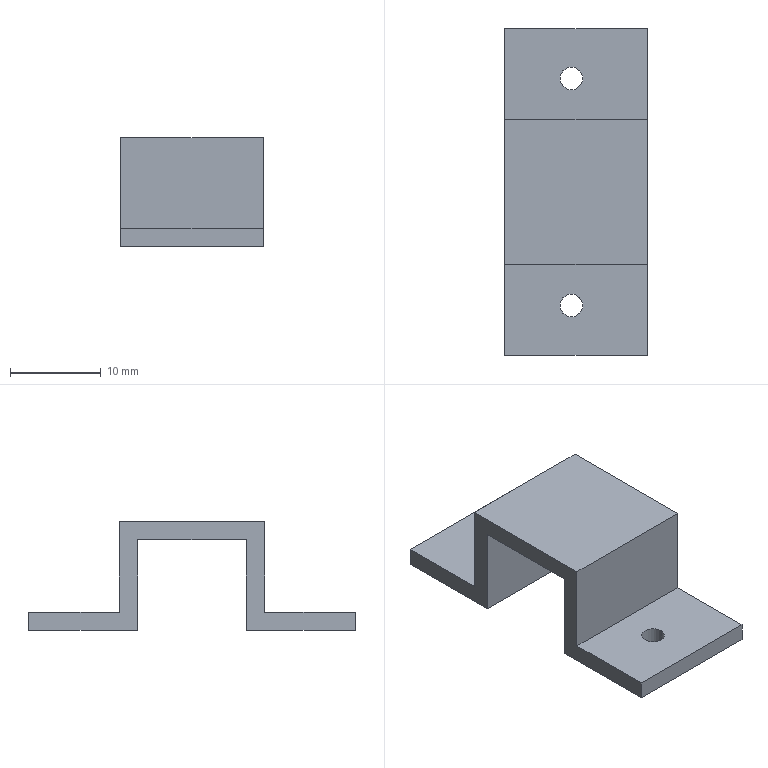Part | SolidWorks | features ICE 3, Extrusion 1, HoleWzd 1 | 1 solid | 18 faces | box 15.7 x 36 x 12 mm | volume 1739 mm3 | plane 14 | cylinder 4 | commonest cylinder face diameters 2.5 x4
STEP:
#1=CARTESIAN_POINT('',(1.25,-12.5,-10.));
#2=VERTEX_POINT('',#1);
#3=CARTESIAN_POINT('',(-1.25,-12.5,-10.));
#4=VERTEX_POINT('',#3);
#5=CARTESIAN_POINT('',(0.,-12.5,-10.));
#6=DIRECTION('',(0.,0.,-1.));
#7=DIRECTION('',(-1.,0.,0.));
#8=AXIS2_PLACEMENT_3D('',#5,#6,#7);
#9=CIRCLE('',#8,1.25);
#10=EDGE_CURVE('',#2,#4,#9,.T.);
#11=ORIENTED_EDGE('',*,*,#10,.T.);
#12=CARTESIAN_POINT('',(-1.25,-12.5,-8.));
#13=VERTEX_POINT('',#12);
#14=CARTESIAN_POINT('',(-1.25,-12.5,-8.));
#15=DIRECTION('',(0.,0.,1.));
#16=VECTOR('',#15,1000.);
#17=LINE('',#14,#16);
#18=EDGE_CURVE('',#4,#13,#17,.T.);
#19=ORIENTED_EDGE('',*,*,#18,.T.);
#20=CARTESIAN_POINT('',(1.25,-12.5,-8.));
#21=VERTEX_POINT('',#20);
#22=CARTESIAN_POINT('',(0.,-12.5,-8.));
#23=DIRECTION('',(0.,0.,1.));
#24=DIRECTION('',(1.,0.,0.));
#25=AXIS2_PLACEMENT_3D('',#22,#23,#24);
#26=CIRCLE('',#25,1.25);
#27=EDGE_CURVE('',#13,#21,#26,.T.);
#28=ORIENTED_EDGE('',*,*,#27,.T.);
#29=CARTESIAN_POINT('',(1.25,-12.5,-8.));
#30=DIRECTION('',(0.,0.,1.));
#31=VECTOR('',#30,1000.);
#32=LINE('',#29,#31);
#33=EDGE_CURVE('',#2,#21,#32,.T.);
#34=ORIENTED_EDGE('',*,*,#33,.F.);
#35=EDGE_LOOP('',(#11,#19,#28,#34));
#36=FACE_OUTER_BOUND('',#35,.T.);
#37=CARTESIAN_POINT('',(0.,-12.5,-8.));
#38=DIRECTION('',(0.,0.,1.));
#39=DIRECTION('',(1.,0.,0.));
#40=AXIS2_PLACEMENT_3D('',#37,#38,#39);
#41=CYLINDRICAL_SURFACE('',#40,1.25);
#42=ADVANCED_FACE('',(#36),#41,.F.);
#43=CARTESIAN_POINT('',(-1.25,12.5,-10.));
#44=VERTEX_POINT('',#43);
#45=CARTESIAN_POINT('',(1.25,12.5,-10.));
#46=VERTEX_POINT('',#45);
#47=CARTESIAN_POINT('',(0.,12.5,-10.));
#48=DIRECTION('',(0.,0.,1.));
#49=DIRECTION('',(1.,0.,0.));
#50=AXIS2_PLACEMENT_3D('',#47,#48,#49);
#51=CIRCLE('',#50,1.25);
#52=EDGE_CURVE('',#44,#46,#51,.T.);
#53=ORIENTED_EDGE('',*,*,#52,.F.);
#54=CARTESIAN_POINT('',(-1.25,12.5,-8.));
#55=VERTEX_POINT('',#54);
#56=CARTESIAN_POINT('',(-1.25,12.5,-8.));
#57=DIRECTION('',(0.,0.,1.));
#58=VECTOR('',#57,1000.);
#59=LINE('',#56,#58);
#60=EDGE_CURVE('',#44,#55,#59,.T.);
#61=ORIENTED_EDGE('',*,*,#60,.T.);
#62=CARTESIAN_POINT('',(1.25,12.5,-8.));
#63=VERTEX_POINT('',#62);
#64=CARTESIAN_POINT('',(0.,12.5,-8.));
#65=DIRECTION('',(0.,0.,1.));
#66=DIRECTION('',(1.,0.,0.));
#67=AXIS2_PLACEMENT_3D('',#64,#65,#66);
#68=CIRCLE('',#67,1.25);
#69=EDGE_CURVE('',#55,#63,#68,.T.);
#70=ORIENTED_EDGE('',*,*,#69,.T.);
#71=CARTESIAN_POINT('',(1.25,12.5,-8.));
#72=DIRECTION('',(0.,0.,1.));
#73=VECTOR('',#72,1000.);
#74=LINE('',#71,#73);
#75=EDGE_CURVE('',#46,#63,#74,.T.);
#76=ORIENTED_EDGE('',*,*,#75,.F.);
#77=EDGE_LOOP('',(#53,#61,#70,#76));
#78=FACE_OUTER_BOUND('',#77,.T.);
#79=CARTESIAN_POINT('',(0.,12.5,-8.));
#80=DIRECTION('',(0.,0.,1.));
#81=DIRECTION('',(1.,0.,0.));
#82=AXIS2_PLACEMENT_3D('',#79,#80,#81);
#83=CYLINDRICAL_SURFACE('',#82,1.25);
#84=ADVANCED_FACE('',(#78),#83,.F.);
#85=CARTESIAN_POINT('',(-7.35,8.,2.));
#86=VERTEX_POINT('',#85);
#87=CARTESIAN_POINT('',(-7.35,8.,-8.));
#88=VERTEX_POINT('',#87);
#89=CARTESIAN_POINT('',(-7.35,8.,2.));
#90=DIRECTION('',(0.,0.,-1.));
#91=VECTOR('',#90,1000.);
#92=LINE('',#89,#91);
#93=EDGE_CURVE('',#86,#88,#92,.T.);
#94=ORIENTED_EDGE('',*,*,#93,.F.);
#95=CARTESIAN_POINT('',(8.35,8.,2.));
#96=VERTEX_POINT('',#95);
#97=CARTESIAN_POINT('',(8.35,8.,2.));
#98=DIRECTION('',(-1.,0.,0.));
#99=VECTOR('',#98,1000.);
#100=LINE('',#97,#99);
#101=EDGE_CURVE('',#96,#86,#100,.T.);
#102=ORIENTED_EDGE('',*,*,#101,.F.);
#103=CARTESIAN_POINT('',(8.35,8.,-8.));
#104=VERTEX_POINT('',#103);
#105=CARTESIAN_POINT('',(8.35,8.,-10.));
#106=DIRECTION('',(0.,0.,1.));
#107=VECTOR('',#106,1000.);
#108=LINE('',#105,#107);
#109=EDGE_CURVE('',#104,#96,#108,.T.);
#110=ORIENTED_EDGE('',*,*,#109,.F.);
#111=CARTESIAN_POINT('',(18.548,8.,-8.));
#112=DIRECTION('',(-1.,0.,0.));
#113=VECTOR('',#112,1000.);
#114=LINE('',#111,#113);
#115=EDGE_CURVE('',#104,#88,#114,.T.);
#116=ORIENTED_EDGE('',*,*,#115,.T.);
#117=EDGE_LOOP('',(#94,#102,#110,#116));
#118=FACE_OUTER_BOUND('',#117,.T.);
#119=CARTESIAN_POINT('',(8.35,8.,-10.));
#120=DIRECTION('',(0.,1.,0.));
#121=DIRECTION('',(0.,0.,1.));
#122=AXIS2_PLACEMENT_3D('',#119,#120,#121);
#123=PLANE('',#122);
#124=ADVANCED_FACE('',(#118),#123,.T.);
#125=CARTESIAN_POINT('',(8.35,-6.,0.));
#126=VERTEX_POINT('',#125);
#127=CARTESIAN_POINT('',(8.35,6.,0.));
#128=VERTEX_POINT('',#127);
#129=CARTESIAN_POINT('',(8.35,6.,0.));
#130=DIRECTION('',(0.,1.,0.));
#131=VECTOR('',#130,1000.);
#132=LINE('',#129,#131);
#133=EDGE_CURVE('',#126,#128,#132,.T.);
#134=ORIENTED_EDGE('',*,*,#133,.T.);
#135=CARTESIAN_POINT('',(8.35,6.,-10.));
#136=VERTEX_POINT('',#135);
#137=CARTESIAN_POINT('',(8.35,6.,-10.));
#138=DIRECTION('',(0.,0.,1.));
#139=VECTOR('',#138,1000.);
#140=LINE('',#137,#139);
#141=EDGE_CURVE('',#136,#128,#140,.T.);
#142=ORIENTED_EDGE('',*,*,#141,.F.);
#143=CARTESIAN_POINT('',(8.35,18.,-10.));
#144=VERTEX_POINT('',#143);
#145=CARTESIAN_POINT('',(8.35,6.,-10.));
#146=DIRECTION('',(0.,1.,0.));
#147=VECTOR('',#146,1000.);
#148=LINE('',#145,#147);
#149=EDGE_CURVE('',#136,#144,#148,.T.);
#150=ORIENTED_EDGE('',*,*,#149,.T.);
#151=CARTESIAN_POINT('',(8.35,18.,-8.));
#152=VERTEX_POINT('',#151);
#153=CARTESIAN_POINT('',(8.35,18.,-10.));
#154=DIRECTION('',(0.,0.,1.));
#155=VECTOR('',#154,1000.);
#156=LINE('',#153,#155);
#157=EDGE_CURVE('',#144,#152,#156,.T.);
#158=ORIENTED_EDGE('',*,*,#157,.T.);
#159=CARTESIAN_POINT('',(8.35,18.,-8.));
#160=DIRECTION('',(0.,-1.,0.));
#161=VECTOR('',#160,1000.);
#162=LINE('',#159,#161);
#163=EDGE_CURVE('',#152,#104,#162,.T.);
#164=ORIENTED_EDGE('',*,*,#163,.T.);
#165=ORIENTED_EDGE('',*,*,#109,.T.);
#166=CARTESIAN_POINT('',(8.35,-8.,2.));
#167=VERTEX_POINT('',#166);
#168=CARTESIAN_POINT('',(8.35,6.,2.));
#169=DIRECTION('',(0.,1.,0.));
#170=VECTOR('',#169,1000.);
#171=LINE('',#168,#170);
#172=EDGE_CURVE('',#167,#96,#171,.T.);
#173=ORIENTED_EDGE('',*,*,#172,.F.);
#174=CARTESIAN_POINT('',(8.35,-8.,-8.));
#175=VERTEX_POINT('',#174);
#176=CARTESIAN_POINT('',(8.35,-8.,-10.));
#177=DIRECTION('',(0.,0.,1.));
#178=VECTOR('',#177,1000.);
#179=LINE('',#176,#178);
#180=EDGE_CURVE('',#175,#167,#179,.T.);
#181=ORIENTED_EDGE('',*,*,#180,.F.);
#182=CARTESIAN_POINT('',(8.35,-18.,-8.));
#183=VERTEX_POINT('',#182);
#184=CARTESIAN_POINT('',(8.35,-18.,-8.));
#185=DIRECTION('',(0.,-1.,0.));
#186=VECTOR('',#185,1000.);
#187=LINE('',#184,#186);
#188=EDGE_CURVE('',#175,#183,#187,.T.);
#189=ORIENTED_EDGE('',*,*,#188,.T.);
#190=CARTESIAN_POINT('',(8.35,-18.,-10.));
#191=VERTEX_POINT('',#190);
#192=CARTESIAN_POINT('',(8.35,-18.,-10.));
#193=DIRECTION('',(0.,0.,-1.));
#194=VECTOR('',#193,1000.);
#195=LINE('',#192,#194);
#196=EDGE_CURVE('',#183,#191,#195,.T.);
#197=ORIENTED_EDGE('',*,*,#196,.T.);
#198=CARTESIAN_POINT('',(8.35,-6.,-10.));
#199=VERTEX_POINT('',#198);
#200=CARTESIAN_POINT('',(8.35,-6.,-10.));
#201=DIRECTION('',(0.,1.,0.));
#202=VECTOR('',#201,1000.);
#203=LINE('',#200,#202);
#204=EDGE_CURVE('',#191,#199,#203,.T.);
#205=ORIENTED_EDGE('',*,*,#204,.T.);
#206=CARTESIAN_POINT('',(8.35,-6.,-10.));
#207=DIRECTION('',(0.,0.,1.));
#208=VECTOR('',#207,1000.);
#209=LINE('',#206,#208);
#210=EDGE_CURVE('',#199,#126,#209,.T.);
#211=ORIENTED_EDGE('',*,*,#210,.T.);
#212=EDGE_LOOP('',(#134,#142,#150,#158,#164,#165,#173,#181,#189,#197,#205,#211));
#213=FACE_OUTER_BOUND('',#212,.T.);
#214=CARTESIAN_POINT('',(8.35,6.,2.));
#215=DIRECTION('',(-1.,0.,0.));
#216=DIRECTION('',(0.,0.,1.));
#217=AXIS2_PLACEMENT_3D('',#214,#215,#216);
#218=PLANE('',#217);
#219=ADVANCED_FACE('',(#213),#218,.F.);
#220=CARTESIAN_POINT('',(-7.35,-8.,2.));
#221=VERTEX_POINT('',#220);
#222=CARTESIAN_POINT('',(-7.35,-8.,2.));
#223=DIRECTION('',(0.,1.,0.));
#224=VECTOR('',#223,1000.);
#225=LINE('',#222,#224);
#226=EDGE_CURVE('',#221,#86,#225,.T.);
#227=ORIENTED_EDGE('',*,*,#226,.F.);
#228=CARTESIAN_POINT('',(8.35,-8.,2.));
#229=DIRECTION('',(1.,0.,0.));
#230=VECTOR('',#229,1000.);
#231=LINE('',#228,#230);
#232=EDGE_CURVE('',#221,#167,#231,.T.);
#233=ORIENTED_EDGE('',*,*,#232,.T.);
#234=ORIENTED_EDGE('',*,*,#172,.T.);
#235=ORIENTED_EDGE('',*,*,#101,.T.);
#236=EDGE_LOOP('',(#227,#233,#234,#235));
#237=FACE_OUTER_BOUND('',#236,.T.);
#238=CARTESIAN_POINT('',(0.,0.,2.));
#239=DIRECTION('',(0.,0.,1.));
#240=DIRECTION('',(1.,0.,0.));
#241=AXIS2_PLACEMENT_3D('',#238,#239,#240);
#242=PLANE('',#241);
#243=ADVANCED_FACE('',(#237),#242,.T.);
#244=CARTESIAN_POINT('',(-7.35,-6.,0.));
#245=VERTEX_POINT('',#244);
#246=CARTESIAN_POINT('',(-8.35,-6.,0.));
#247=DIRECTION('',(1.,0.,0.));
#248=VECTOR('',#247,1000.);
#249=LINE('',#246,#248);
#250=EDGE_CURVE('',#245,#126,#249,.T.);
#251=ORIENTED_EDGE('',*,*,#250,.F.);
#252=CARTESIAN_POINT('',(-7.35,6.,0.));
#253=VERTEX_POINT('',#252);
#254=CARTESIAN_POINT('',(-7.35,6.,0.));
#255=DIRECTION('',(0.,-1.,0.));
#256=VECTOR('',#255,1000.);
#257=LINE('',#254,#256);
#258=EDGE_CURVE('',#253,#245,#257,.T.);
#259=ORIENTED_EDGE('',*,*,#258,.F.);
#260=CARTESIAN_POINT('',(-8.35,6.,0.));
#261=DIRECTION('',(-1.,0.,0.));
#262=VECTOR('',#261,1000.);
#263=LINE('',#260,#262);
#264=EDGE_CURVE('',#128,#253,#263,.T.);
#265=ORIENTED_EDGE('',*,*,#264,.F.);
#266=ORIENTED_EDGE('',*,*,#133,.F.);
#267=EDGE_LOOP('',(#251,#259,#265,#266));
#268=FACE_OUTER_BOUND('',#267,.T.);
#269=CARTESIAN_POINT('',(0.,0.,0.));
#270=DIRECTION('',(0.,0.,1.));
#271=DIRECTION('',(1.,0.,0.));
#272=AXIS2_PLACEMENT_3D('',#269,#270,#271);
#273=PLANE('',#272);
#274=ADVANCED_FACE('',(#268),#273,.F.);
#275=CARTESIAN_POINT('',(-7.35,6.,-10.));
#276=VERTEX_POINT('',#275);
#277=CARTESIAN_POINT('',(-7.35,6.,-10.));
#278=DIRECTION('',(0.,0.,1.));
#279=VECTOR('',#278,1000.);
#280=LINE('',#277,#279);
#281=EDGE_CURVE('',#276,#253,#280,.T.);
#282=ORIENTED_EDGE('',*,*,#281,.F.);
#283=CARTESIAN_POINT('',(-8.35,6.,-10.));
#284=DIRECTION('',(1.,0.,0.));
#285=VECTOR('',#284,1000.);
#286=LINE('',#283,#285);
#287=EDGE_CURVE('',#276,#136,#286,.T.);
#288=ORIENTED_EDGE('',*,*,#287,.T.);
#289=ORIENTED_EDGE('',*,*,#141,.T.);
#290=ORIENTED_EDGE('',*,*,#264,.T.);
#291=EDGE_LOOP('',(#282,#288,#289,#290));
#292=FACE_OUTER_BOUND('',#291,.T.);
#293=CARTESIAN_POINT('',(-8.35,6.,-10.));
#294=DIRECTION('',(0.,-1.,0.));
#295=DIRECTION('',(0.,0.,-1.));
#296=AXIS2_PLACEMENT_3D('',#293,#294,#295);
#297=PLANE('',#296);
#298=ADVANCED_FACE('',(#292),#297,.T.);
#299=CARTESIAN_POINT('',(0.,12.5,-10.));
#300=DIRECTION('',(0.,0.,1.));
#301=DIRECTION('',(1.,0.,0.));
#302=AXIS2_PLACEMENT_3D('',#299,#300,#301);
#303=CIRCLE('',#302,1.25);
#304=EDGE_CURVE('',#46,#44,#303,.T.);
#305=ORIENTED_EDGE('',*,*,#304,.T.);
#306=ORIENTED_EDGE('',*,*,#52,.T.);
#307=EDGE_LOOP('',(#305,#306));
#308=FACE_BOUND('',#307,.T.);
#309=ORIENTED_EDGE('',*,*,#287,.F.);
#310=CARTESIAN_POINT('',(-7.35,18.,-10.));
#311=VERTEX_POINT('',#310);
#312=CARTESIAN_POINT('',(-7.35,18.,-10.));
#313=DIRECTION('',(0.,-1.,0.));
#314=VECTOR('',#313,1000.);
#315=LINE('',#312,#314);
#316=EDGE_CURVE('',#311,#276,#315,.T.);
#317=ORIENTED_EDGE('',*,*,#316,.F.);
#318=CARTESIAN_POINT('',(18.548,18.,-10.));
#319=DIRECTION('',(-1.,0.,0.));
#320=VECTOR('',#319,1000.);
#321=LINE('',#318,#320);
#322=EDGE_CURVE('',#144,#311,#321,.T.);
#323=ORIENTED_EDGE('',*,*,#322,.F.);
#324=ORIENTED_EDGE('',*,*,#149,.F.);
#325=EDGE_LOOP('',(#309,#317,#323,#324));
#326=FACE_OUTER_BOUND('',#325,.T.);
#327=CARTESIAN_POINT('',(0.,0.,-10.));
#328=DIRECTION('',(0.,0.,1.));
#329=DIRECTION('',(1.,0.,0.));
#330=AXIS2_PLACEMENT_3D('',#327,#328,#329);
#331=PLANE('',#330);
#332=ADVANCED_FACE('',(#308,#326),#331,.F.);
#333=CARTESIAN_POINT('',(-7.35,-8.,-8.));
#334=VERTEX_POINT('',#333);
#335=CARTESIAN_POINT('',(-7.35,-8.,-8.));
#336=DIRECTION('',(0.,0.,1.));
#337=VECTOR('',#336,1000.);
#338=LINE('',#335,#337);
#339=EDGE_CURVE('',#334,#221,#338,.T.);
#340=ORIENTED_EDGE('',*,*,#339,.F.);
#341=CARTESIAN_POINT('',(18.548,-8.,-8.));
#342=DIRECTION('',(-1.,0.,0.));
#343=VECTOR('',#342,1000.);
#344=LINE('',#341,#343);
#345=EDGE_CURVE('',#175,#334,#344,.T.);
#346=ORIENTED_EDGE('',*,*,#345,.F.);
#347=ORIENTED_EDGE('',*,*,#180,.T.);
#348=ORIENTED_EDGE('',*,*,#232,.F.);
#349=EDGE_LOOP('',(#340,#346,#347,#348));
#350=FACE_OUTER_BOUND('',#349,.T.);
#351=CARTESIAN_POINT('',(8.35,-8.,-10.));
#352=DIRECTION('',(0.,-1.,0.));
#353=DIRECTION('',(0.,0.,-1.));
#354=AXIS2_PLACEMENT_3D('',#351,#352,#353);
#355=PLANE('',#354);
#356=ADVANCED_FACE('',(#350),#355,.T.);
#357=CARTESIAN_POINT('',(-7.35,-6.,-10.));
#358=VERTEX_POINT('',#357);
#359=CARTESIAN_POINT('',(-7.35,-6.,0.));
#360=DIRECTION('',(0.,0.,-1.));
#361=VECTOR('',#360,1000.);
#362=LINE('',#359,#361);
#363=EDGE_CURVE('',#245,#358,#362,.T.);
#364=ORIENTED_EDGE('',*,*,#363,.F.);
#365=ORIENTED_EDGE('',*,*,#250,.T.);
#366=ORIENTED_EDGE('',*,*,#210,.F.);
#367=CARTESIAN_POINT('',(-8.35,-6.,-10.));
#368=DIRECTION('',(-1.,0.,0.));
#369=VECTOR('',#368,1000.);
#370=LINE('',#367,#369);
#371=EDGE_CURVE('',#199,#358,#370,.T.);
#372=ORIENTED_EDGE('',*,*,#371,.T.);
#373=EDGE_LOOP('',(#364,#365,#366,#372));
#374=FACE_OUTER_BOUND('',#373,.T.);
#375=CARTESIAN_POINT('',(-8.35,-6.,-10.));
#376=DIRECTION('',(0.,1.,0.));
#377=DIRECTION('',(0.,0.,1.));
#378=AXIS2_PLACEMENT_3D('',#375,#376,#377);
#379=PLANE('',#378);
#380=ADVANCED_FACE('',(#374),#379,.T.);
#381=CARTESIAN_POINT('',(-7.35,-18.,-10.));
#382=VERTEX_POINT('',#381);
#383=CARTESIAN_POINT('',(-7.35,-6.,-10.));
#384=DIRECTION('',(0.,-1.,0.));
#385=VECTOR('',#384,1000.);
#386=LINE('',#383,#385);
#387=EDGE_CURVE('',#358,#382,#386,.T.);
#388=ORIENTED_EDGE('',*,*,#387,.F.);
#389=ORIENTED_EDGE('',*,*,#371,.F.);
#390=ORIENTED_EDGE('',*,*,#204,.F.);
#391=CARTESIAN_POINT('',(18.548,-18.,-10.));
#392=DIRECTION('',(-1.,0.,0.));
#393=VECTOR('',#392,1000.);
#394=LINE('',#391,#393);
#395=EDGE_CURVE('',#191,#382,#394,.T.);
#396=ORIENTED_EDGE('',*,*,#395,.T.);
#397=EDGE_LOOP('',(#388,#389,#390,#396));
#398=FACE_OUTER_BOUND('',#397,.T.);
#399=ORIENTED_EDGE('',*,*,#10,.F.);
#400=CARTESIAN_POINT('',(0.,-12.5,-10.));
#401=DIRECTION('',(0.,0.,-1.));
#402=DIRECTION('',(-1.,0.,0.));
#403=AXIS2_PLACEMENT_3D('',#400,#401,#402);
#404=CIRCLE('',#403,1.25);
#405=EDGE_CURVE('',#4,#2,#404,.T.);
#406=ORIENTED_EDGE('',*,*,#405,.F.);
#407=EDGE_LOOP('',(#399,#406));
#408=FACE_BOUND('',#407,.T.);
#409=CARTESIAN_POINT('',(0.,0.,-10.));
#410=DIRECTION('',(0.,0.,-1.));
#411=DIRECTION('',(-1.,0.,0.));
#412=AXIS2_PLACEMENT_3D('',#409,#410,#411);
#413=PLANE('',#412);
#414=ADVANCED_FACE('',(#398,#408),#413,.T.);
#415=CARTESIAN_POINT('',(-7.35,-18.,-8.));
#416=VERTEX_POINT('',#415);
#417=CARTESIAN_POINT('',(-7.35,-18.,-8.));
#418=DIRECTION('',(0.,1.,0.));
#419=VECTOR('',#418,1000.);
#420=LINE('',#417,#419);
#421=EDGE_CURVE('',#416,#334,#420,.T.);
#422=ORIENTED_EDGE('',*,*,#421,.F.);
#423=CARTESIAN_POINT('',(18.548,-18.,-8.));
#424=DIRECTION('',(-1.,0.,0.));
#425=VECTOR('',#424,1000.);
#426=LINE('',#423,#425);
#427=EDGE_CURVE('',#183,#416,#426,.T.);
#428=ORIENTED_EDGE('',*,*,#427,.F.);
#429=ORIENTED_EDGE('',*,*,#188,.F.);
#430=ORIENTED_EDGE('',*,*,#345,.T.);
#431=EDGE_LOOP('',(#422,#428,#429,#430));
#432=FACE_OUTER_BOUND('',#431,.T.);
#433=CARTESIAN_POINT('',(0.,-12.5,-8.));
#434=DIRECTION('',(0.,0.,1.));
#435=DIRECTION('',(1.,0.,0.));
#436=AXIS2_PLACEMENT_3D('',#433,#434,#435);
#437=CIRCLE('',#436,1.25);
#438=EDGE_CURVE('',#21,#13,#437,.T.);
#439=ORIENTED_EDGE('',*,*,#438,.F.);
#440=ORIENTED_EDGE('',*,*,#27,.F.);
#441=EDGE_LOOP('',(#439,#440));
#442=FACE_BOUND('',#441,.T.);
#443=CARTESIAN_POINT('',(18.548,-18.,-8.));
#444=DIRECTION('',(0.,0.,1.));
#445=DIRECTION('',(1.,0.,0.));
#446=AXIS2_PLACEMENT_3D('',#443,#444,#445);
#447=PLANE('',#446);
#448=ADVANCED_FACE('',(#432,#442),#447,.T.);
#449=CARTESIAN_POINT('',(-7.35,-18.,-10.));
#450=DIRECTION('',(0.,0.,1.));
#451=VECTOR('',#450,1000.);
#452=LINE('',#449,#451);
#453=EDGE_CURVE('',#382,#416,#452,.T.);
#454=ORIENTED_EDGE('',*,*,#453,.F.);
#455=ORIENTED_EDGE('',*,*,#395,.F.);
#456=ORIENTED_EDGE('',*,*,#196,.F.);
#457=ORIENTED_EDGE('',*,*,#427,.T.);
#458=EDGE_LOOP('',(#454,#455,#456,#457));
#459=FACE_OUTER_BOUND('',#458,.T.);
#460=CARTESIAN_POINT('',(18.548,-18.,-10.));
#461=DIRECTION('',(0.,-1.,0.));
#462=DIRECTION('',(0.,0.,-1.));
#463=AXIS2_PLACEMENT_3D('',#460,#461,#462);
#464=PLANE('',#463);
#465=ADVANCED_FACE('',(#459),#464,.T.);
#466=CARTESIAN_POINT('',(-7.35,18.,-8.));
#467=VERTEX_POINT('',#466);
#468=CARTESIAN_POINT('',(-7.35,18.,-8.));
#469=DIRECTION('',(0.,0.,-1.));
#470=VECTOR('',#469,1000.);
#471=LINE('',#468,#470);
#472=EDGE_CURVE('',#467,#311,#471,.T.);
#473=ORIENTED_EDGE('',*,*,#472,.F.);
#474=CARTESIAN_POINT('',(18.548,18.,-8.));
#475=DIRECTION('',(-1.,0.,0.));
#476=VECTOR('',#475,1000.);
#477=LINE('',#474,#476);
#478=EDGE_CURVE('',#152,#467,#477,.T.);
#479=ORIENTED_EDGE('',*,*,#478,.F.);
#480=ORIENTED_EDGE('',*,*,#157,.F.);
#481=ORIENTED_EDGE('',*,*,#322,.T.);
#482=EDGE_LOOP('',(#473,#479,#480,#481));
#483=FACE_OUTER_BOUND('',#482,.T.);
#484=CARTESIAN_POINT('',(18.548,18.,-10.));
#485=DIRECTION('',(0.,1.,0.));
#486=DIRECTION('',(0.,0.,1.));
#487=AXIS2_PLACEMENT_3D('',#484,#485,#486);
#488=PLANE('',#487);
#489=ADVANCED_FACE('',(#483),#488,.T.);
#490=CARTESIAN_POINT('',(-7.35,8.,-8.));
#491=DIRECTION('',(0.,1.,0.));
#492=VECTOR('',#491,1000.);
#493=LINE('',#490,#492);
#494=EDGE_CURVE('',#88,#467,#493,.T.);
#495=ORIENTED_EDGE('',*,*,#494,.F.);
#496=ORIENTED_EDGE('',*,*,#115,.F.);
#497=ORIENTED_EDGE('',*,*,#163,.F.);
#498=ORIENTED_EDGE('',*,*,#478,.T.);
#499=EDGE_LOOP('',(#495,#496,#497,#498));
#500=FACE_OUTER_BOUND('',#499,.T.);
#501=CARTESIAN_POINT('',(0.,12.5,-8.));
#502=DIRECTION('',(0.,0.,1.));
#503=DIRECTION('',(1.,0.,0.));
#504=AXIS2_PLACEMENT_3D('',#501,#502,#503);
#505=CIRCLE('',#504,1.25);
#506=EDGE_CURVE('',#63,#55,#505,.T.);
#507=ORIENTED_EDGE('',*,*,#506,.F.);
#508=ORIENTED_EDGE('',*,*,#69,.F.);
#509=EDGE_LOOP('',(#507,#508));
#510=FACE_BOUND('',#509,.T.);
#511=CARTESIAN_POINT('',(18.548,18.,-8.));
#512=DIRECTION('',(0.,0.,1.));
#513=DIRECTION('',(1.,0.,0.));
#514=AXIS2_PLACEMENT_3D('',#511,#512,#513);
#515=PLANE('',#514);
#516=ADVANCED_FACE('',(#500,#510),#515,.T.);
#517=ORIENTED_EDGE('',*,*,#60,.F.);
#518=ORIENTED_EDGE('',*,*,#304,.F.);
#519=ORIENTED_EDGE('',*,*,#75,.T.);
#520=ORIENTED_EDGE('',*,*,#506,.T.);
#521=EDGE_LOOP('',(#517,#518,#519,#520));
#522=FACE_OUTER_BOUND('',#521,.T.);
#523=CARTESIAN_POINT('',(0.,12.5,-8.));
#524=DIRECTION('',(0.,0.,1.));
#525=DIRECTION('',(1.,0.,0.));
#526=AXIS2_PLACEMENT_3D('',#523,#524,#525);
#527=CYLINDRICAL_SURFACE('',#526,1.25);
#528=ADVANCED_FACE('',(#522),#527,.F.);
#529=ORIENTED_EDGE('',*,*,#18,.F.);
#530=ORIENTED_EDGE('',*,*,#405,.T.);
#531=ORIENTED_EDGE('',*,*,#33,.T.);
#532=ORIENTED_EDGE('',*,*,#438,.T.);
#533=EDGE_LOOP('',(#529,#530,#531,#532));
#534=FACE_OUTER_BOUND('',#533,.T.);
#535=CARTESIAN_POINT('',(0.,-12.5,-8.));
#536=DIRECTION('',(0.,0.,1.));
#537=DIRECTION('',(1.,0.,0.));
#538=AXIS2_PLACEMENT_3D('',#535,#536,#537);
#539=CYLINDRICAL_SURFACE('',#538,1.25);
#540=ADVANCED_FACE('',(#534),#539,.F.);
#541=ORIENTED_EDGE('',*,*,#281,.T.);
#542=ORIENTED_EDGE('',*,*,#258,.T.);
#543=ORIENTED_EDGE('',*,*,#363,.T.);
#544=ORIENTED_EDGE('',*,*,#387,.T.);
#545=ORIENTED_EDGE('',*,*,#453,.T.);
#546=ORIENTED_EDGE('',*,*,#421,.T.);
#547=ORIENTED_EDGE('',*,*,#339,.T.);
#548=ORIENTED_EDGE('',*,*,#226,.T.);
#549=ORIENTED_EDGE('',*,*,#93,.T.);
#550=ORIENTED_EDGE('',*,*,#494,.T.);
#551=ORIENTED_EDGE('',*,*,#472,.T.);
#552=ORIENTED_EDGE('',*,*,#316,.T.);
#553=EDGE_LOOP('',(#541,#542,#543,#544,#545,#546,#547,#548,#549,#550,#551,#552));
#554=FACE_OUTER_BOUND('',#553,.T.);
#555=CARTESIAN_POINT('',(-7.35,0.,0.));
#556=DIRECTION('',(1.,0.,0.));
#557=DIRECTION('',(0.,0.,-1.));
#558=AXIS2_PLACEMENT_3D('',#555,#556,#557);
#559=PLANE('',#558);
#560=ADVANCED_FACE('',(#554),#559,.F.);
#561=CLOSED_SHELL('',(#42,#84,#124,#219,#243,#274,#298,#332,#356,#380,#414,#448,#465,#489,#516,#528,#540,#560));
#562=MANIFOLD_SOLID_BREP('',#561);
#563=CARTESIAN_POINT('',(0.,0.,0.));
#564=DIRECTION('',(0.,0.,1.));
#565=DIRECTION('',(1.,0.,0.));
#566=AXIS2_PLACEMENT_3D('',#563,#564,#565);
#567=(LENGTH_UNIT()NAMED_UNIT(*)SI_UNIT(.MILLI.,.METRE.));
#568=UNCERTAINTY_MEASURE_WITH_UNIT(LENGTH_MEASURE(0.00001),#567,'','');
#569=(NAMED_UNIT(*)PLANE_ANGLE_UNIT()SI_UNIT($,.RADIAN.));
#570=(NAMED_UNIT(*)SI_UNIT($,.STERADIAN.)SOLID_ANGLE_UNIT());
#571=(GEOMETRIC_REPRESENTATION_CONTEXT(3)GLOBAL_UNCERTAINTY_ASSIGNED_CONTEXT((#568))GLOBAL_UNIT_ASSIGNED_CONTEXT((#567,#569,#570))REPRESENTATION_CONTEXT('',''));
#572=ADVANCED_BREP_SHAPE_REPRESENTATION('',(#562,#566),#571);